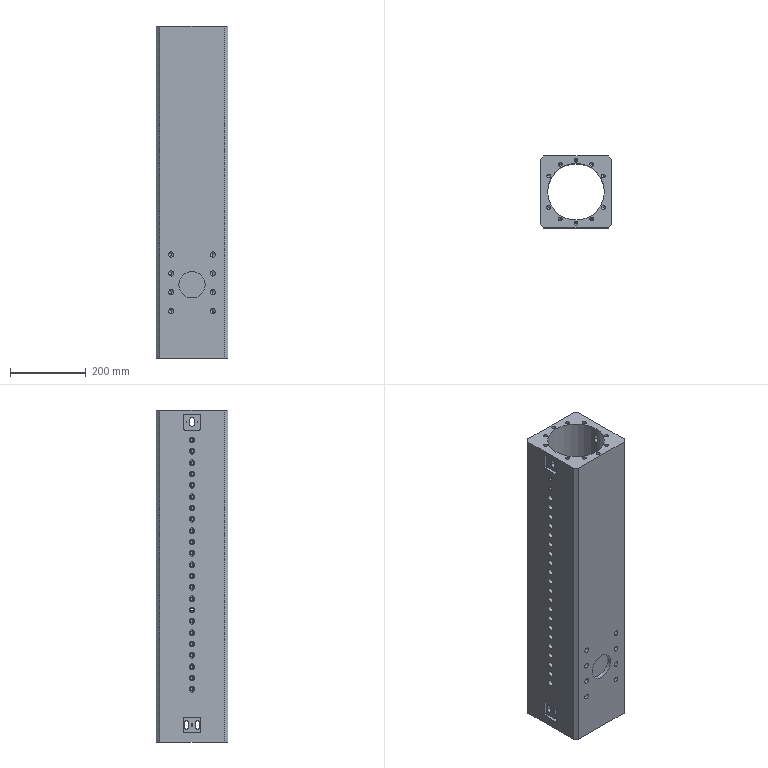Part | SolidWorks | features ICE 10, HoleWzd 8, Chamfer 4, Fillet 2, LPattern 2, MirrorPattern 2, CirPattern 1, Extrusion 1 | 1 solid | 339 faces | box 190 x 190 x 879 mm | volume 15737206 mm3 | cylinder 214 | plane 69 | cone 56 | commonest cylinder face diameters 9 x52 15 x46 10.2 x40 13 x18 2.5 x16 6 x16